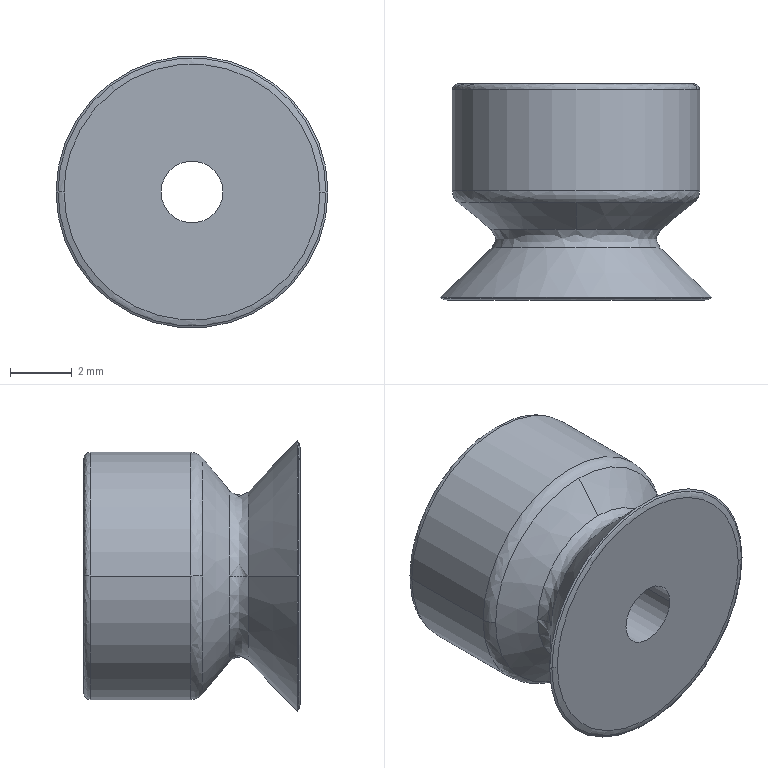Part | STEP file | 11-_ZP2-B08MUN_PADC11 | 1 solid | 20 faces | box 8.8 x 7 x 8.8 mm | volume 283.623 mm3 | spline 8 | cone 6 | cylinder 4 | plane 2 | commonest cylinder face diameters 2 x2 8 x2
STEP:
#1=CARTESIAN_POINT('',(0.,3.15,-3.815));
#2=VERTEX_POINT('',#1);
#3=CARTESIAN_POINT('',(-3.815,3.15,0.));
#4=VERTEX_POINT('',#3);
#5=CARTESIAN_POINT('',(0.,3.15,0.));
#6=DIRECTION('',(0.,1.,0.));
#7=DIRECTION('',(1.,0.,0.));
#8=AXIS2_PLACEMENT_3D('',#5,#6,#7);
#9=CIRCLE('',#8,3.815);
#10=EDGE_CURVE('',#2,#4,#9,.T.);
#11=ORIENTED_EDGE('',*,*,#10,.T.);
#12=CARTESIAN_POINT('',(-4.,3.538,0.));
#13=VERTEX_POINT('',#12);
#14=CARTESIAN_POINT('',(-3.5,3.538,0.));
#15=DIRECTION('',(0.,0.,-1.));
#16=DIRECTION('',(-1.,0.,0.));
#17=AXIS2_PLACEMENT_3D('',#14,#15,#16);
#18=CIRCLE('',#17,0.5);
#19=EDGE_CURVE('',#4,#13,#18,.T.);
#20=ORIENTED_EDGE('',*,*,#19,.T.);
#21=CARTESIAN_POINT('',(4.,3.538,0.));
#22=VERTEX_POINT('',#21);
#23=CARTESIAN_POINT('',(0.,3.538,0.));
#24=DIRECTION('',(0.,1.,0.));
#25=DIRECTION('',(-1.,0.,0.));
#26=AXIS2_PLACEMENT_3D('',#23,#24,#25);
#27=CIRCLE('',#26,4.);
#28=EDGE_CURVE('',#22,#13,#27,.T.);
#29=ORIENTED_EDGE('',*,*,#28,.F.);
#30=CARTESIAN_POINT('',(3.815,3.15,0.));
#31=VERTEX_POINT('',#30);
#32=CARTESIAN_POINT('',(3.5,3.538,0.));
#33=DIRECTION('',(0.,0.,1.));
#34=DIRECTION('',(1.,0.,0.));
#35=AXIS2_PLACEMENT_3D('',#32,#33,#34);
#36=CIRCLE('',#35,0.5);
#37=EDGE_CURVE('',#31,#22,#36,.T.);
#38=ORIENTED_EDGE('',*,*,#37,.F.);
#39=CARTESIAN_POINT('',(0.,3.15,0.));
#40=DIRECTION('',(0.,1.,0.));
#41=DIRECTION('',(1.,0.,0.));
#42=AXIS2_PLACEMENT_3D('',#39,#40,#41);
#43=CIRCLE('',#42,3.815);
#44=EDGE_CURVE('',#31,#2,#43,.T.);
#45=ORIENTED_EDGE('',*,*,#44,.T.);
#46=EDGE_LOOP('',(#11,#20,#29,#38,#45));
#47=FACE_OUTER_BOUND('',#46,.T.);
#48=CARTESIAN_POINT('',(-3.815,3.15,0.));
#49=CARTESIAN_POINT('',(-3.815,3.15,-7.631));
#50=CARTESIAN_POINT('',(3.815,3.15,-7.631));
#51=CARTESIAN_POINT('',(3.815,3.15,0.));
#52=CARTESIAN_POINT('',(-3.934,3.247,0.));
#53=CARTESIAN_POINT('',(-3.934,3.247,-7.868));
#54=CARTESIAN_POINT('',(3.934,3.247,-7.868));
#55=CARTESIAN_POINT('',(3.934,3.247,0.));
#56=CARTESIAN_POINT('',(-4.,3.385,0.));
#57=CARTESIAN_POINT('',(-4.,3.385,-8.));
#58=CARTESIAN_POINT('',(4.,3.385,-8.));
#59=CARTESIAN_POINT('',(4.,3.385,0.));
#60=CARTESIAN_POINT('',(-4.,3.538,0.));
#61=CARTESIAN_POINT('',(-4.,3.538,-8.));
#62=CARTESIAN_POINT('',(4.,3.538,-8.));
#63=CARTESIAN_POINT('',(4.,3.538,0.));
#64=(BOUNDED_SURFACE()B_SPLINE_SURFACE(3,3,((#48,#49,#50,#51),(#52,#53,#54,#55),(#56,#57,#58,#59),(#60,#61,#62,#63)),.UNSPECIFIED.,.F.,.F.,.F.)B_SPLINE_SURFACE_WITH_KNOTS((4,4),(4,4),(0.,1.),(0.,1.),.UNSPECIFIED.)GEOMETRIC_REPRESENTATION_ITEM()RATIONAL_B_SPLINE_SURFACE(((1.,0.3333,0.3333,1.),(0.9353,0.3118,0.3118,0.9353),(0.9353,0.3118,0.3118,0.9353),(1.,0.3333,0.3333,1.)))REPRESENTATION_ITEM('')SURFACE());
#65=ADVANCED_FACE('',(#47),#64,.T.);
#66=CARTESIAN_POINT('',(-4.,6.8,0.));
#67=VERTEX_POINT('',#66);
#68=CARTESIAN_POINT('',(4.,6.8,0.));
#69=VERTEX_POINT('',#68);
#70=CARTESIAN_POINT('',(0.,6.8,0.));
#71=DIRECTION('',(0.,-1.,0.));
#72=DIRECTION('',(-1.,0.,0.));
#73=AXIS2_PLACEMENT_3D('',#70,#71,#72);
#74=CIRCLE('',#73,4.);
#75=EDGE_CURVE('',#67,#69,#74,.T.);
#76=ORIENTED_EDGE('',*,*,#75,.F.);
#77=CARTESIAN_POINT('',(-3.8,7.,0.));
#78=VERTEX_POINT('',#77);
#79=CARTESIAN_POINT('',(-3.8,6.8,0.));
#80=DIRECTION('',(0.,0.,-1.));
#81=DIRECTION('',(-1.,0.,0.));
#82=AXIS2_PLACEMENT_3D('',#79,#80,#81);
#83=CIRCLE('',#82,0.2);
#84=EDGE_CURVE('',#67,#78,#83,.T.);
#85=ORIENTED_EDGE('',*,*,#84,.T.);
#86=CARTESIAN_POINT('',(3.8,7.,0.));
#87=VERTEX_POINT('',#86);
#88=CARTESIAN_POINT('',(-3.8,7.,0.));
#89=CARTESIAN_POINT('',(-3.8,7.,-7.6));
#90=CARTESIAN_POINT('',(3.8,7.,-7.6));
#91=CARTESIAN_POINT('',(3.8,7.,0.));
#92=(BOUNDED_CURVE()B_SPLINE_CURVE(3,(#88,#89,#90,#91),.UNSPECIFIED.,.F.,.F.)B_SPLINE_CURVE_WITH_KNOTS((4,4),(0.5,1.),.UNSPECIFIED.)CURVE()GEOMETRIC_REPRESENTATION_ITEM()RATIONAL_B_SPLINE_CURVE((1.,0.3333,0.3333,1.))REPRESENTATION_ITEM(''));
#93=EDGE_CURVE('',#78,#87,#92,.T.);
#94=ORIENTED_EDGE('',*,*,#93,.T.);
#95=CARTESIAN_POINT('',(3.8,6.8,0.));
#96=DIRECTION('',(0.,0.,1.));
#97=DIRECTION('',(1.,0.,0.));
#98=AXIS2_PLACEMENT_3D('',#95,#96,#97);
#99=CIRCLE('',#98,0.2);
#100=EDGE_CURVE('',#69,#87,#99,.T.);
#101=ORIENTED_EDGE('',*,*,#100,.F.);
#102=EDGE_LOOP('',(#76,#85,#94,#101));
#103=FACE_OUTER_BOUND('',#102,.T.);
#104=CARTESIAN_POINT('',(-4.,6.8,0.));
#105=CARTESIAN_POINT('',(-4.,6.8,-8.));
#106=CARTESIAN_POINT('',(4.,6.8,-8.));
#107=CARTESIAN_POINT('',(4.,6.8,0.));
#108=CARTESIAN_POINT('',(-4.,6.917,0.));
#109=CARTESIAN_POINT('',(-4.,6.917,-8.));
#110=CARTESIAN_POINT('',(4.,6.917,-8.));
#111=CARTESIAN_POINT('',(4.,6.917,0.));
#112=CARTESIAN_POINT('',(-3.917,7.,0.));
#113=CARTESIAN_POINT('',(-3.917,7.,-7.834));
#114=CARTESIAN_POINT('',(3.917,7.,-7.834));
#115=CARTESIAN_POINT('',(3.917,7.,0.));
#116=CARTESIAN_POINT('',(-3.8,7.,0.));
#117=CARTESIAN_POINT('',(-3.8,7.,-7.6));
#118=CARTESIAN_POINT('',(3.8,7.,-7.6));
#119=CARTESIAN_POINT('',(3.8,7.,0.));
#120=(BOUNDED_SURFACE()B_SPLINE_SURFACE(3,3,((#104,#105,#106,#107),(#108,#109,#110,#111),(#112,#113,#114,#115),(#116,#117,#118,#119)),.UNSPECIFIED.,.F.,.F.,.F.)B_SPLINE_SURFACE_WITH_KNOTS((4,4),(4,4),(0.,1.),(0.,1.),.UNSPECIFIED.)GEOMETRIC_REPRESENTATION_ITEM()RATIONAL_B_SPLINE_SURFACE(((1.,0.3333,0.3333,1.),(0.8047,0.2682,0.2682,0.8047),(0.8047,0.2682,0.2682,0.8047),(1.,0.3333,0.3333,1.)))REPRESENTATION_ITEM('')SURFACE());
#121=ADVANCED_FACE('',(#103),#120,.T.);
#122=CARTESIAN_POINT('',(-2.752,2.286,0.));
#123=VERTEX_POINT('',#122);
#124=CARTESIAN_POINT('',(0.,2.286,2.752));
#125=VERTEX_POINT('',#124);
#126=CARTESIAN_POINT('',(0.,2.286,0.));
#127=DIRECTION('',(0.,1.,0.));
#128=DIRECTION('',(-1.,0.,0.));
#129=AXIS2_PLACEMENT_3D('',#126,#127,#128);
#130=CIRCLE('',#129,2.752);
#131=EDGE_CURVE('',#123,#125,#130,.T.);
#132=ORIENTED_EDGE('',*,*,#131,.F.);
#133=CARTESIAN_POINT('',(-2.728,1.687,0.));
#134=VERTEX_POINT('',#133);
#135=CARTESIAN_POINT('',(-3.005,1.976,0.));
#136=DIRECTION('',(0.,0.,-1.));
#137=DIRECTION('',(-1.,0.,0.));
#138=AXIS2_PLACEMENT_3D('',#135,#136,#137);
#139=CIRCLE('',#138,0.4);
#140=EDGE_CURVE('',#123,#134,#139,.T.);
#141=ORIENTED_EDGE('',*,*,#140,.T.);
#142=CARTESIAN_POINT('',(2.728,1.687,0.));
#143=VERTEX_POINT('',#142);
#144=CARTESIAN_POINT('',(0.,1.687,0.));
#145=DIRECTION('',(0.,-1.,0.));
#146=DIRECTION('',(1.,0.,0.));
#147=AXIS2_PLACEMENT_3D('',#144,#145,#146);
#148=CIRCLE('',#147,2.728);
#149=EDGE_CURVE('',#143,#134,#148,.T.);
#150=ORIENTED_EDGE('',*,*,#149,.F.);
#151=CARTESIAN_POINT('',(2.752,2.286,0.));
#152=VERTEX_POINT('',#151);
#153=CARTESIAN_POINT('',(3.005,1.976,0.));
#154=DIRECTION('',(0.,0.,1.));
#155=DIRECTION('',(1.,0.,0.));
#156=AXIS2_PLACEMENT_3D('',#153,#154,#155);
#157=CIRCLE('',#156,0.4);
#158=EDGE_CURVE('',#152,#143,#157,.T.);
#159=ORIENTED_EDGE('',*,*,#158,.F.);
#160=CARTESIAN_POINT('',(0.,2.286,0.));
#161=DIRECTION('',(0.,1.,0.));
#162=DIRECTION('',(-1.,0.,0.));
#163=AXIS2_PLACEMENT_3D('',#160,#161,#162);
#164=CIRCLE('',#163,2.752);
#165=EDGE_CURVE('',#125,#152,#164,.T.);
#166=ORIENTED_EDGE('',*,*,#165,.F.);
#167=EDGE_LOOP('',(#132,#141,#150,#159,#166));
#168=FACE_OUTER_BOUND('',#167,.T.);
#169=CARTESIAN_POINT('',(2.752,2.286,0.));
#170=CARTESIAN_POINT('',(2.752,2.286,5.505));
#171=CARTESIAN_POINT('',(-2.752,2.286,5.505));
#172=CARTESIAN_POINT('',(-2.752,2.286,0.));
#173=CARTESIAN_POINT('',(2.552,2.123,0.));
#174=CARTESIAN_POINT('',(2.552,2.123,5.103));
#175=CARTESIAN_POINT('',(-2.552,2.123,5.103));
#176=CARTESIAN_POINT('',(-2.552,2.123,0.));
#177=CARTESIAN_POINT('',(2.541,1.865,0.));
#178=CARTESIAN_POINT('',(2.541,1.865,5.083));
#179=CARTESIAN_POINT('',(-2.541,1.865,5.083));
#180=CARTESIAN_POINT('',(-2.541,1.865,0.));
#181=CARTESIAN_POINT('',(2.728,1.687,0.));
#182=CARTESIAN_POINT('',(2.728,1.687,5.457));
#183=CARTESIAN_POINT('',(-2.728,1.687,5.457));
#184=CARTESIAN_POINT('',(-2.728,1.687,0.));
#185=(BOUNDED_SURFACE()B_SPLINE_SURFACE(3,3,((#169,#170,#171,#172),(#173,#174,#175,#176),(#177,#178,#179,#180),(#181,#182,#183,#184)),.UNSPECIFIED.,.F.,.F.,.F.)B_SPLINE_SURFACE_WITH_KNOTS((4,4),(4,4),(0.,1.),(0.,1.),.UNSPECIFIED.)GEOMETRIC_REPRESENTATION_ITEM()RATIONAL_B_SPLINE_SURFACE(((1.,0.3333,0.3333,1.),(0.7741,0.258,0.258,0.7741),(0.7741,0.258,0.258,0.7741),(1.,0.3333,0.3333,1.)))REPRESENTATION_ITEM('')SURFACE());
#186=ADVANCED_FACE('',(#168),#185,.F.);
#187=CARTESIAN_POINT('',(-4.137,0.,0.));
#188=VERTEX_POINT('',#187);
#189=CARTESIAN_POINT('',(4.137,0.,0.));
#190=VERTEX_POINT('',#189);
#191=CARTESIAN_POINT('',(-4.137,0.,0.));
#192=CARTESIAN_POINT('',(-4.137,0.,-0.2629));
#193=CARTESIAN_POINT('',(-4.101,0.,-0.6503));
#194=CARTESIAN_POINT('',(-3.995,0.,-1.091));
#195=CARTESIAN_POINT('',(-3.926,0.,-1.308));
#196=CARTESIAN_POINT('',(-3.893,0.,-1.4));
#197=CARTESIAN_POINT('',(-3.87,0.,-1.462));
#198=CARTESIAN_POINT('',(-3.859,0.,-1.49));
#199=CARTESIAN_POINT('',(-3.795,0.,-1.653));
#200=CARTESIAN_POINT('',(-3.709,0.,-1.843));
#201=CARTESIAN_POINT('',(-3.608,0.,-2.025));
#202=CARTESIAN_POINT('',(-3.538,0.,-2.146));
#203=CARTESIAN_POINT('',(-3.502,0.,-2.204));
#204=CARTESIAN_POINT('',(-3.307,0.,-2.503));
#205=CARTESIAN_POINT('',(-3.127,0.,-2.724));
#206=CARTESIAN_POINT('',(-2.824,0.,-3.026));
#207=CARTESIAN_POINT('',(-2.666,0.,-3.169));
#208=CARTESIAN_POINT('',(-2.497,0.,-3.299));
#209=CARTESIAN_POINT('',(-2.382,0.,-3.383));
#210=CARTESIAN_POINT('',(-2.322,0.,-3.424));
#211=CARTESIAN_POINT('',(-2.147,0.,-3.539));
#212=CARTESIAN_POINT('',(-1.967,0.,-3.644));
#213=CARTESIAN_POINT('',(-1.748,0.,-3.751));
#214=CARTESIAN_POINT('',(-1.652,0.,-3.793));
#215=CARTESIAN_POINT('',(-1.588,0.,-3.82));
#216=CARTESIAN_POINT('',(-1.553,0.,-3.834));
#217=CARTESIAN_POINT('',(-1.034,0.,-4.04));
#218=CARTESIAN_POINT('',(-0.5257,0.,-4.137));
#219=CARTESIAN_POINT('',(0.2629,0.,-4.137));
#220=CARTESIAN_POINT('',(0.6503,0.,-4.101));
#221=CARTESIAN_POINT('',(1.091,0.,-3.995));
#222=CARTESIAN_POINT('',(1.308,0.,-3.926));
#223=CARTESIAN_POINT('',(1.4,0.,-3.893));
#224=CARTESIAN_POINT('',(1.462,0.,-3.87));
#225=CARTESIAN_POINT('',(1.49,0.,-3.859));
#226=CARTESIAN_POINT('',(1.653,0.,-3.795));
#227=CARTESIAN_POINT('',(1.843,0.,-3.709));
#228=CARTESIAN_POINT('',(2.025,0.,-3.608));
#229=CARTESIAN_POINT('',(2.146,0.,-3.538));
#230=CARTESIAN_POINT('',(2.204,0.,-3.502));
#231=CARTESIAN_POINT('',(2.503,0.,-3.307));
#232=CARTESIAN_POINT('',(2.724,0.,-3.127));
#233=CARTESIAN_POINT('',(3.026,0.,-2.824));
#234=CARTESIAN_POINT('',(3.169,0.,-2.666));
#235=CARTESIAN_POINT('',(3.299,0.,-2.497));
#236=CARTESIAN_POINT('',(3.383,0.,-2.382));
#237=CARTESIAN_POINT('',(3.424,0.,-2.322));
#238=CARTESIAN_POINT('',(3.539,0.,-2.147));
#239=CARTESIAN_POINT('',(3.644,0.,-1.967));
#240=CARTESIAN_POINT('',(3.751,0.,-1.748));
#241=CARTESIAN_POINT('',(3.793,0.,-1.652));
#242=CARTESIAN_POINT('',(3.82,0.,-1.588));
#243=CARTESIAN_POINT('',(3.834,0.,-1.553));
#244=CARTESIAN_POINT('',(4.04,0.,-1.034));
#245=CARTESIAN_POINT('',(4.137,0.,-0.5262));
#246=CARTESIAN_POINT('',(4.137,0.,0.));
#247=B_SPLINE_CURVE_WITH_KNOTS('',3,(#191,#192,#193,#194,#195,#196,#197,#198,#199,#200,#201,#202,#203,#204,#205,#206,#207,#208,#209,#210,#211,#212,#213,#214,#215,#216,#217,#218,#219,#220,#221,#222,#223,#224,#225,#226,#227,#228,#229,#230,#231,#232,#233,#234,#235,#236,#237,#238,#239,#240,#241,#242,#243,#244,#245,#246),.UNSPECIFIED.,.F.,.F.,(4,1,1,1,2,2,1,2,2,2,1,2,2,1,1,2,2,2,1,1,1,2,2,1,2,2,2,1,2,2,1,1,2,2,4),(0.5,0.5313,0.5469,0.5547,0.5586,0.5625,0.5781,0.5859,0.5938,0.625,0.6406,0.6484,0.6562,0.6719,0.6797,0.6836,0.6875,0.75,0.7813,0.7969,0.8047,0.8086,0.8125,0.8281,0.8359,0.8438,0.875,0.8906,0.8984,0.9063,0.9219,0.9297,0.9336,0.9375,1.),.UNSPECIFIED.);
#248=EDGE_CURVE('',#188,#190,#247,.T.);
#249=ORIENTED_EDGE('',*,*,#248,.F.);
#250=CARTESIAN_POINT('',(-4.337,0.05359,0.));
#251=VERTEX_POINT('',#250);
#252=CARTESIAN_POINT('',(-4.137,0.4,0.));
#253=DIRECTION('',(0.,0.,-1.));
#254=DIRECTION('',(-1.,0.,0.));
#255=AXIS2_PLACEMENT_3D('',#252,#253,#254);
#256=CIRCLE('',#255,0.4);
#257=EDGE_CURVE('',#188,#251,#256,.T.);
#258=ORIENTED_EDGE('',*,*,#257,.T.);
#259=CARTESIAN_POINT('',(4.337,0.05359,0.));
#260=VERTEX_POINT('',#259);
#261=CARTESIAN_POINT('',(0.,0.05359,0.));
#262=DIRECTION('',(0.,1.,0.));
#263=DIRECTION('',(-1.,0.,0.));
#264=AXIS2_PLACEMENT_3D('',#261,#262,#263);
#265=CIRCLE('',#264,4.337);
#266=EDGE_CURVE('',#260,#251,#265,.T.);
#267=ORIENTED_EDGE('',*,*,#266,.F.);
#268=CARTESIAN_POINT('',(4.137,0.4,0.));
#269=DIRECTION('',(0.,0.,1.));
#270=DIRECTION('',(1.,0.,0.));
#271=AXIS2_PLACEMENT_3D('',#268,#269,#270);
#272=CIRCLE('',#271,0.4);
#273=EDGE_CURVE('',#190,#260,#272,.T.);
#274=ORIENTED_EDGE('',*,*,#273,.F.);
#275=EDGE_LOOP('',(#249,#258,#267,#274));
#276=FACE_OUTER_BOUND('',#275,.T.);
#277=CARTESIAN_POINT('',(-4.137,0.,0.));
#278=CARTESIAN_POINT('',(-4.137,0.,-8.274));
#279=CARTESIAN_POINT('',(4.137,0.,-8.274));
#280=CARTESIAN_POINT('',(4.137,0.,0.));
#281=CARTESIAN_POINT('',(-4.208,0.,0.));
#282=CARTESIAN_POINT('',(-4.208,0.,-8.415));
#283=CARTESIAN_POINT('',(4.208,0.,-8.415));
#284=CARTESIAN_POINT('',(4.208,0.,0.));
#285=CARTESIAN_POINT('',(-4.276,0.01828,0.));
#286=CARTESIAN_POINT('',(-4.276,0.01828,-8.552));
#287=CARTESIAN_POINT('',(4.276,0.01828,-8.552));
#288=CARTESIAN_POINT('',(4.276,0.01828,0.));
#289=CARTESIAN_POINT('',(-4.337,0.05359,0.));
#290=CARTESIAN_POINT('',(-4.337,0.05359,-8.674));
#291=CARTESIAN_POINT('',(4.337,0.05359,-8.674));
#292=CARTESIAN_POINT('',(4.337,0.05359,0.));
#293=(BOUNDED_SURFACE()B_SPLINE_SURFACE(3,3,((#277,#278,#279,#280),(#281,#282,#283,#284),(#285,#286,#287,#288),(#289,#290,#291,#292)),.UNSPECIFIED.,.F.,.F.,.F.)B_SPLINE_SURFACE_WITH_KNOTS((4,4),(4,4),(0.,1.),(0.,1.),.UNSPECIFIED.)GEOMETRIC_REPRESENTATION_ITEM()RATIONAL_B_SPLINE_SURFACE(((1.,0.3333,0.3333,1.),(0.9773,0.3258,0.3258,0.9773),(0.9773,0.3258,0.3258,0.9773),(1.,0.3333,0.3333,1.)))REPRESENTATION_ITEM('')SURFACE());
#294=ADVANCED_FACE('',(#276),#293,.T.);
#295=CARTESIAN_POINT('',(0.,3.538,0.));
#296=DIRECTION('',(0.,1.,0.));
#297=DIRECTION('',(-1.,0.,0.));
#298=AXIS2_PLACEMENT_3D('',#295,#296,#297);
#299=CIRCLE('',#298,4.);
#300=EDGE_CURVE('',#13,#22,#299,.T.);
#301=ORIENTED_EDGE('',*,*,#300,.T.);
#302=CARTESIAN_POINT('',(4.,0.,0.));
#303=DIRECTION('',(0.,1.,0.));
#304=VECTOR('',#303,1000.);
#305=LINE('',#302,#304);
#306=EDGE_CURVE('',#22,#69,#305,.T.);
#307=ORIENTED_EDGE('',*,*,#306,.T.);
#308=CARTESIAN_POINT('',(0.,6.8,0.));
#309=DIRECTION('',(0.,-1.,0.));
#310=DIRECTION('',(-1.,0.,0.));
#311=AXIS2_PLACEMENT_3D('',#308,#309,#310);
#312=CIRCLE('',#311,4.);
#313=EDGE_CURVE('',#69,#67,#312,.T.);
#314=ORIENTED_EDGE('',*,*,#313,.T.);
#315=CARTESIAN_POINT('',(-4.,0.,0.));
#316=DIRECTION('',(0.,1.,0.));
#317=VECTOR('',#316,1000.);
#318=LINE('',#315,#317);
#319=EDGE_CURVE('',#13,#67,#318,.T.);
#320=ORIENTED_EDGE('',*,*,#319,.F.);
#321=EDGE_LOOP('',(#301,#307,#314,#320));
#322=FACE_OUTER_BOUND('',#321,.T.);
#323=CARTESIAN_POINT('',(0.,0.,0.));
#324=DIRECTION('',(0.,1.,0.));
#325=DIRECTION('',(-1.,0.,0.));
#326=AXIS2_PLACEMENT_3D('',#323,#324,#325);
#327=CYLINDRICAL_SURFACE('',#326,4.);
#328=ADVANCED_FACE('',(#322),#327,.T.);
#329=ORIENTED_EDGE('',*,*,#165,.T.);
#330=CARTESIAN_POINT('',(0.,2.286,-2.752));
#331=VERTEX_POINT('',#330);
#332=CARTESIAN_POINT('',(0.,2.286,0.));
#333=DIRECTION('',(0.,1.,0.));
#334=DIRECTION('',(-1.,0.,0.));
#335=AXIS2_PLACEMENT_3D('',#332,#333,#334);
#336=CIRCLE('',#335,2.752);
#337=EDGE_CURVE('',#152,#331,#336,.T.);
#338=ORIENTED_EDGE('',*,*,#337,.T.);
#339=CARTESIAN_POINT('',(0.,3.15,-3.815));
#340=DIRECTION('',(0.,0.6306,-0.7761));
#341=VECTOR('',#340,1000.);
#342=LINE('',#339,#341);
#343=EDGE_CURVE('',#331,#2,#342,.T.);
#344=ORIENTED_EDGE('',*,*,#343,.T.);
#345=ORIENTED_EDGE('',*,*,#44,.F.);
#346=CARTESIAN_POINT('',(0.,3.15,3.815));
#347=VERTEX_POINT('',#346);
#348=CARTESIAN_POINT('',(0.,3.15,0.));
#349=DIRECTION('',(0.,1.,0.));
#350=DIRECTION('',(1.,0.,0.));
#351=AXIS2_PLACEMENT_3D('',#348,#349,#350);
#352=CIRCLE('',#351,3.815);
#353=EDGE_CURVE('',#347,#31,#352,.T.);
#354=ORIENTED_EDGE('',*,*,#353,.F.);
#355=CARTESIAN_POINT('',(0.,3.15,3.815));
#356=DIRECTION('',(0.,0.6306,0.7761));
#357=VECTOR('',#356,1000.);
#358=LINE('',#355,#357);
#359=EDGE_CURVE('',#125,#347,#358,.T.);
#360=ORIENTED_EDGE('',*,*,#359,.F.);
#361=EDGE_LOOP('',(#329,#338,#344,#345,#354,#360));
#362=FACE_OUTER_BOUND('',#361,.T.);
#363=CARTESIAN_POINT('',(0.,3.15,0.));
#364=DIRECTION('',(0.,1.,0.));
#365=DIRECTION('',(0.,0.,1.));
#366=AXIS2_PLACEMENT_3D('',#363,#364,#365);
#367=CONICAL_SURFACE('',#366,3.815,0.8885);
#368=ADVANCED_FACE('',(#362),#367,.T.);
#369=CARTESIAN_POINT('',(1.,0.,0.));
#370=VERTEX_POINT('',#369);
#371=CARTESIAN_POINT('',(-1.,0.,0.));
#372=VERTEX_POINT('',#371);
#373=CARTESIAN_POINT('',(0.,0.,0.));
#374=DIRECTION('',(0.,1.,0.));
#375=DIRECTION('',(-1.,0.,0.));
#376=AXIS2_PLACEMENT_3D('',#373,#374,#375);
#377=CIRCLE('',#376,1.);
#378=EDGE_CURVE('',#370,#372,#377,.T.);
#379=ORIENTED_EDGE('',*,*,#378,.F.);
#380=CARTESIAN_POINT('',(1.,7.,0.));
#381=VERTEX_POINT('',#380);
#382=CARTESIAN_POINT('',(1.,0.,0.));
#383=DIRECTION('',(0.,1.,0.));
#384=VECTOR('',#383,1000.);
#385=LINE('',#382,#384);
#386=EDGE_CURVE('',#370,#381,#385,.T.);
#387=ORIENTED_EDGE('',*,*,#386,.T.);
#388=CARTESIAN_POINT('',(-1.,7.,0.));
#389=VERTEX_POINT('',#388);
#390=CARTESIAN_POINT('',(0.,7.,0.));
#391=DIRECTION('',(0.,-1.,0.));
#392=DIRECTION('',(-1.,0.,0.));
#393=AXIS2_PLACEMENT_3D('',#390,#391,#392);
#394=CIRCLE('',#393,1.);
#395=EDGE_CURVE('',#389,#381,#394,.T.);
#396=ORIENTED_EDGE('',*,*,#395,.F.);
#397=CARTESIAN_POINT('',(-1.,0.,0.));
#398=DIRECTION('',(0.,1.,0.));
#399=VECTOR('',#398,1000.);
#400=LINE('',#397,#399);
#401=EDGE_CURVE('',#372,#389,#400,.T.);
#402=ORIENTED_EDGE('',*,*,#401,.F.);
#403=EDGE_LOOP('',(#379,#387,#396,#402));
#404=FACE_OUTER_BOUND('',#403,.T.);
#405=CARTESIAN_POINT('',(0.,0.,0.));
#406=DIRECTION('',(0.,1.,0.));
#407=DIRECTION('',(-1.,0.,0.));
#408=AXIS2_PLACEMENT_3D('',#405,#406,#407);
#409=CYLINDRICAL_SURFACE('',#408,1.);
#410=ADVANCED_FACE('',(#404),#409,.F.);
#411=ORIENTED_EDGE('',*,*,#149,.T.);
#412=CARTESIAN_POINT('',(-4.4,0.09,0.));
#413=VERTEX_POINT('',#412);
#414=CARTESIAN_POINT('',(-4.4,0.09,0.));
#415=DIRECTION('',(-0.7232,-0.6906,0.));
#416=VECTOR('',#415,1000.);
#417=LINE('',#414,#416);
#418=EDGE_CURVE('',#134,#413,#417,.T.);
#419=ORIENTED_EDGE('',*,*,#418,.T.);
#420=CARTESIAN_POINT('',(4.4,0.09,0.));
#421=VERTEX_POINT('',#420);
#422=CARTESIAN_POINT('',(0.,0.09,0.));
#423=DIRECTION('',(0.,1.,0.));
#424=DIRECTION('',(1.,0.,0.));
#425=AXIS2_PLACEMENT_3D('',#422,#423,#424);
#426=CIRCLE('',#425,4.4);
#427=EDGE_CURVE('',#413,#421,#426,.T.);
#428=ORIENTED_EDGE('',*,*,#427,.T.);
#429=CARTESIAN_POINT('',(4.4,0.09,0.));
#430=DIRECTION('',(0.7232,-0.6906,0.));
#431=VECTOR('',#430,1000.);
#432=LINE('',#429,#431);
#433=EDGE_CURVE('',#143,#421,#432,.T.);
#434=ORIENTED_EDGE('',*,*,#433,.F.);
#435=EDGE_LOOP('',(#411,#419,#428,#434));
#436=FACE_OUTER_BOUND('',#435,.T.);
#437=CARTESIAN_POINT('',(0.,0.09,0.));
#438=DIRECTION('',(0.,-1.,0.));
#439=DIRECTION('',(1.,0.,0.));
#440=AXIS2_PLACEMENT_3D('',#437,#438,#439);
#441=CONICAL_SURFACE('',#440,4.4,0.8084);
#442=ADVANCED_FACE('',(#436),#441,.T.);
#443=CARTESIAN_POINT('',(0.,0.05359,0.));
#444=DIRECTION('',(0.,1.,0.));
#445=DIRECTION('',(-1.,0.,0.));
#446=AXIS2_PLACEMENT_3D('',#443,#444,#445);
#447=CIRCLE('',#446,4.337);
#448=EDGE_CURVE('',#251,#260,#447,.T.);
#449=ORIENTED_EDGE('',*,*,#448,.T.);
#450=CARTESIAN_POINT('',(4.4,0.09,0.));
#451=DIRECTION('',(0.866,0.5,0.));
#452=VECTOR('',#451,1000.);
#453=LINE('',#450,#452);
#454=EDGE_CURVE('',#260,#421,#453,.T.);
#455=ORIENTED_EDGE('',*,*,#454,.T.);
#456=ORIENTED_EDGE('',*,*,#427,.F.);
#457=CARTESIAN_POINT('',(-4.4,0.09,0.));
#458=DIRECTION('',(-0.866,0.5,0.));
#459=VECTOR('',#458,1000.);
#460=LINE('',#457,#459);
#461=EDGE_CURVE('',#251,#413,#460,.T.);
#462=ORIENTED_EDGE('',*,*,#461,.F.);
#463=EDGE_LOOP('',(#449,#455,#456,#462));
#464=FACE_OUTER_BOUND('',#463,.T.);
#465=CARTESIAN_POINT('',(0.,0.09,0.));
#466=DIRECTION('',(0.,1.,0.));
#467=DIRECTION('',(-1.,0.,0.));
#468=AXIS2_PLACEMENT_3D('',#465,#466,#467);
#469=CONICAL_SURFACE('',#468,4.4,1.047);
#470=ADVANCED_FACE('',(#464),#469,.T.);
#471=ORIENTED_EDGE('',*,*,#306,.F.);
#472=ORIENTED_EDGE('',*,*,#28,.T.);
#473=ORIENTED_EDGE('',*,*,#319,.T.);
#474=ORIENTED_EDGE('',*,*,#75,.T.);
#475=EDGE_LOOP('',(#471,#472,#473,#474));
#476=FACE_OUTER_BOUND('',#475,.T.);
#477=CARTESIAN_POINT('',(0.,0.,0.));
#478=DIRECTION('',(0.,1.,0.));
#479=DIRECTION('',(-1.,0.,0.));
#480=AXIS2_PLACEMENT_3D('',#477,#478,#479);
#481=CYLINDRICAL_SURFACE('',#480,4.);
#482=ADVANCED_FACE('',(#476),#481,.T.);
#483=ORIENTED_EDGE('',*,*,#19,.F.);
#484=CARTESIAN_POINT('',(0.,3.15,0.));
#485=DIRECTION('',(0.,1.,0.));
#486=DIRECTION('',(1.,0.,0.));
#487=AXIS2_PLACEMENT_3D('',#484,#485,#486);
#488=CIRCLE('',#487,3.815);
#489=EDGE_CURVE('',#4,#347,#488,.T.);
#490=ORIENTED_EDGE('',*,*,#489,.T.);
#491=ORIENTED_EDGE('',*,*,#353,.T.);
#492=ORIENTED_EDGE('',*,*,#37,.T.);
#493=ORIENTED_EDGE('',*,*,#300,.F.);
#494=EDGE_LOOP('',(#483,#490,#491,#492,#493));
#495=FACE_OUTER_BOUND('',#494,.T.);
#496=CARTESIAN_POINT('',(3.815,3.15,0.));
#497=CARTESIAN_POINT('',(3.815,3.15,7.631));
#498=CARTESIAN_POINT('',(-3.815,3.15,7.631));
#499=CARTESIAN_POINT('',(-3.815,3.15,0.));
#500=CARTESIAN_POINT('',(3.934,3.247,0.));
#501=CARTESIAN_POINT('',(3.934,3.247,7.868));
#502=CARTESIAN_POINT('',(-3.934,3.247,7.868));
#503=CARTESIAN_POINT('',(-3.934,3.247,0.));
#504=CARTESIAN_POINT('',(4.,3.385,0.));
#505=CARTESIAN_POINT('',(4.,3.385,8.));
#506=CARTESIAN_POINT('',(-4.,3.385,8.));
#507=CARTESIAN_POINT('',(-4.,3.385,0.));
#508=CARTESIAN_POINT('',(4.,3.538,0.));
#509=CARTESIAN_POINT('',(4.,3.538,8.));
#510=CARTESIAN_POINT('',(-4.,3.538,8.));
#511=CARTESIAN_POINT('',(-4.,3.538,0.));
#512=(BOUNDED_SURFACE()B_SPLINE_SURFACE(3,3,((#496,#497,#498,#499),(#500,#501,#502,#503),(#504,#505,#506,#507),(#508,#509,#510,#511)),.UNSPECIFIED.,.F.,.F.,.F.)B_SPLINE_SURFACE_WITH_KNOTS((4,4),(4,4),(0.,1.),(0.,1.),.UNSPECIFIED.)GEOMETRIC_REPRESENTATION_ITEM()RATIONAL_B_SPLINE_SURFACE(((1.,0.3333,0.3333,1.),(0.9353,0.3118,0.3118,0.9353),(0.9353,0.3118,0.3118,0.9353),(1.,0.3333,0.3333,1.)))REPRESENTATION_ITEM('')SURFACE());
#513=ADVANCED_FACE('',(#495),#512,.T.);
#514=ORIENTED_EDGE('',*,*,#84,.F.);
#515=ORIENTED_EDGE('',*,*,#313,.F.);
#516=ORIENTED_EDGE('',*,*,#100,.T.);
#517=CARTESIAN_POINT('',(3.8,7.,0.));
#518=CARTESIAN_POINT('',(3.8,7.,7.6));
#519=CARTESIAN_POINT('',(-3.8,7.,7.6));
#520=CARTESIAN_POINT('',(-3.8,7.,0.));
#521=(BOUNDED_CURVE()B_SPLINE_CURVE(3,(#517,#518,#519,#520),.UNSPECIFIED.,.F.,.F.)B_SPLINE_CURVE_WITH_KNOTS((4,4),(0.,0.5),.UNSPECIFIED.)CURVE()GEOMETRIC_REPRESENTATION_ITEM()RATIONAL_B_SPLINE_CURVE((1.,0.3333,0.3333,1.))REPRESENTATION_ITEM(''));
#522=EDGE_CURVE('',#87,#78,#521,.T.);
#523=ORIENTED_EDGE('',*,*,#522,.T.);
#524=EDGE_LOOP('',(#514,#515,#516,#523));
#525=FACE_OUTER_BOUND('',#524,.T.);
#526=CARTESIAN_POINT('',(4.,6.8,0.));
#527=CARTESIAN_POINT('',(4.,6.8,8.));
#528=CARTESIAN_POINT('',(-4.,6.8,8.));
#529=CARTESIAN_POINT('',(-4.,6.8,0.));
#530=CARTESIAN_POINT('',(4.,6.917,0.));
#531=CARTESIAN_POINT('',(4.,6.917,8.));
#532=CARTESIAN_POINT('',(-4.,6.917,8.));
#533=CARTESIAN_POINT('',(-4.,6.917,0.));
#534=CARTESIAN_POINT('',(3.917,7.,0.));
#535=CARTESIAN_POINT('',(3.917,7.,7.834));
#536=CARTESIAN_POINT('',(-3.917,7.,7.834));
#537=CARTESIAN_POINT('',(-3.917,7.,0.));
#538=CARTESIAN_POINT('',(3.8,7.,0.));
#539=CARTESIAN_POINT('',(3.8,7.,7.6));
#540=CARTESIAN_POINT('',(-3.8,7.,7.6));
#541=CARTESIAN_POINT('',(-3.8,7.,0.));
#542=(BOUNDED_SURFACE()B_SPLINE_SURFACE(3,3,((#526,#527,#528,#529),(#530,#531,#532,#533),(#534,#535,#536,#537),(#538,#539,#540,#541)),.UNSPECIFIED.,.F.,.F.,.F.)B_SPLINE_SURFACE_WITH_KNOTS((4,4),(4,4),(0.,1.),(0.,1.),.UNSPECIFIED.)GEOMETRIC_REPRESENTATION_ITEM()RATIONAL_B_SPLINE_SURFACE(((1.,0.3333,0.3333,1.),(0.8047,0.2682,0.2682,0.8047),(0.8047,0.2682,0.2682,0.8047),(1.,0.3333,0.3333,1.)))REPRESENTATION_ITEM('')SURFACE());
#543=ADVANCED_FACE('',(#525),#542,.T.);
#544=ORIENTED_EDGE('',*,*,#343,.F.);
#545=CARTESIAN_POINT('',(0.,2.286,0.));
#546=DIRECTION('',(0.,1.,0.));
#547=DIRECTION('',(-1.,0.,0.));
#548=AXIS2_PLACEMENT_3D('',#545,#546,#547);
#549=CIRCLE('',#548,2.752);
#550=EDGE_CURVE('',#331,#123,#549,.T.);
#551=ORIENTED_EDGE('',*,*,#550,.T.);
#552=ORIENTED_EDGE('',*,*,#131,.T.);
#553=ORIENTED_EDGE('',*,*,#359,.T.);
#554=ORIENTED_EDGE('',*,*,#489,.F.);
#555=ORIENTED_EDGE('',*,*,#10,.F.);
#556=EDGE_LOOP('',(#544,#551,#552,#553,#554,#555));
#557=FACE_OUTER_BOUND('',#556,.T.);
#558=CARTESIAN_POINT('',(0.,3.15,0.));
#559=DIRECTION('',(0.,1.,0.));
#560=DIRECTION('',(0.,0.,1.));
#561=AXIS2_PLACEMENT_3D('',#558,#559,#560);
#562=CONICAL_SURFACE('',#561,3.815,0.8885);
#563=ADVANCED_FACE('',(#557),#562,.T.);
#564=ORIENTED_EDGE('',*,*,#522,.F.);
#565=ORIENTED_EDGE('',*,*,#93,.F.);
#566=EDGE_LOOP('',(#564,#565));
#567=FACE_OUTER_BOUND('',#566,.T.);
#568=ORIENTED_EDGE('',*,*,#395,.T.);
#569=CARTESIAN_POINT('',(0.,7.,0.));
#570=DIRECTION('',(0.,-1.,0.));
#571=DIRECTION('',(-1.,0.,0.));
#572=AXIS2_PLACEMENT_3D('',#569,#570,#571);
#573=CIRCLE('',#572,1.);
#574=EDGE_CURVE('',#381,#389,#573,.T.);
#575=ORIENTED_EDGE('',*,*,#574,.T.);
#576=EDGE_LOOP('',(#568,#575));
#577=FACE_BOUND('',#576,.T.);
#578=CARTESIAN_POINT('',(3.8,7.,0.));
#579=DIRECTION('',(0.,1.,0.));
#580=DIRECTION('',(-1.,0.,0.));
#581=AXIS2_PLACEMENT_3D('',#578,#579,#580);
#582=PLANE('',#581);
#583=ADVANCED_FACE('',(#567,#577),#582,.T.);
#584=ORIENTED_EDGE('',*,*,#140,.F.);
#585=ORIENTED_EDGE('',*,*,#550,.F.);
#586=ORIENTED_EDGE('',*,*,#337,.F.);
#587=ORIENTED_EDGE('',*,*,#158,.T.);
#588=CARTESIAN_POINT('',(0.,1.687,0.));
#589=DIRECTION('',(0.,-1.,0.));
#590=DIRECTION('',(1.,0.,0.));
#591=AXIS2_PLACEMENT_3D('',#588,#589,#590);
#592=CIRCLE('',#591,2.728);
#593=EDGE_CURVE('',#134,#143,#592,.T.);
#594=ORIENTED_EDGE('',*,*,#593,.F.);
#595=EDGE_LOOP('',(#584,#585,#586,#587,#594));
#596=FACE_OUTER_BOUND('',#595,.T.);
#597=CARTESIAN_POINT('',(-2.752,2.286,0.));
#598=CARTESIAN_POINT('',(-2.752,2.286,-5.505));
#599=CARTESIAN_POINT('',(2.752,2.286,-5.505));
#600=CARTESIAN_POINT('',(2.752,2.286,0.));
#601=CARTESIAN_POINT('',(-2.552,2.123,0.));
#602=CARTESIAN_POINT('',(-2.552,2.123,-5.103));
#603=CARTESIAN_POINT('',(2.552,2.123,-5.103));
#604=CARTESIAN_POINT('',(2.552,2.123,0.));
#605=CARTESIAN_POINT('',(-2.541,1.865,0.));
#606=CARTESIAN_POINT('',(-2.541,1.865,-5.083));
#607=CARTESIAN_POINT('',(2.541,1.865,-5.083));
#608=CARTESIAN_POINT('',(2.541,1.865,0.));
#609=CARTESIAN_POINT('',(-2.728,1.687,0.));
#610=CARTESIAN_POINT('',(-2.728,1.687,-5.457));
#611=CARTESIAN_POINT('',(2.728,1.687,-5.457));
#612=CARTESIAN_POINT('',(2.728,1.687,0.));
#613=(BOUNDED_SURFACE()B_SPLINE_SURFACE(3,3,((#597,#598,#599,#600),(#601,#602,#603,#604),(#605,#606,#607,#608),(#609,#610,#611,#612)),.UNSPECIFIED.,.F.,.F.,.F.)B_SPLINE_SURFACE_WITH_KNOTS((4,4),(4,4),(0.,1.),(0.,1.),.UNSPECIFIED.)GEOMETRIC_REPRESENTATION_ITEM()RATIONAL_B_SPLINE_SURFACE(((1.,0.3333,0.3333,1.),(0.7741,0.258,0.258,0.7741),(0.7741,0.258,0.258,0.7741),(1.,0.3333,0.3333,1.)))REPRESENTATION_ITEM('')SURFACE());
#614=ADVANCED_FACE('',(#596),#613,.F.);
#615=ORIENTED_EDGE('',*,*,#386,.F.);
#616=CARTESIAN_POINT('',(0.,0.,0.));
#617=DIRECTION('',(0.,1.,0.));
#618=DIRECTION('',(-1.,0.,0.));
#619=AXIS2_PLACEMENT_3D('',#616,#617,#618);
#620=CIRCLE('',#619,1.);
#621=EDGE_CURVE('',#372,#370,#620,.T.);
#622=ORIENTED_EDGE('',*,*,#621,.F.);
#623=ORIENTED_EDGE('',*,*,#401,.T.);
#624=ORIENTED_EDGE('',*,*,#574,.F.);
#625=EDGE_LOOP('',(#615,#622,#623,#624));
#626=FACE_OUTER_BOUND('',#625,.T.);
#627=CARTESIAN_POINT('',(0.,0.,0.));
#628=DIRECTION('',(0.,1.,0.));
#629=DIRECTION('',(-1.,0.,0.));
#630=AXIS2_PLACEMENT_3D('',#627,#628,#629);
#631=CYLINDRICAL_SURFACE('',#630,1.);
#632=ADVANCED_FACE('',(#626),#631,.F.);
#633=ORIENTED_EDGE('',*,*,#418,.F.);
#634=ORIENTED_EDGE('',*,*,#593,.T.);
#635=ORIENTED_EDGE('',*,*,#433,.T.);
#636=CARTESIAN_POINT('',(0.,0.09,0.));
#637=DIRECTION('',(0.,1.,0.));
#638=DIRECTION('',(1.,0.,0.));
#639=AXIS2_PLACEMENT_3D('',#636,#637,#638);
#640=CIRCLE('',#639,4.4);
#641=EDGE_CURVE('',#421,#413,#640,.T.);
#642=ORIENTED_EDGE('',*,*,#641,.T.);
#643=EDGE_LOOP('',(#633,#634,#635,#642));
#644=FACE_OUTER_BOUND('',#643,.T.);
#645=CARTESIAN_POINT('',(0.,0.09,0.));
#646=DIRECTION('',(0.,-1.,0.));
#647=DIRECTION('',(1.,0.,0.));
#648=AXIS2_PLACEMENT_3D('',#645,#646,#647);
#649=CONICAL_SURFACE('',#648,4.4,0.8084);
#650=ADVANCED_FACE('',(#644),#649,.T.);
#651=ORIENTED_EDGE('',*,*,#621,.T.);
#652=ORIENTED_EDGE('',*,*,#378,.T.);
#653=EDGE_LOOP('',(#651,#652));
#654=FACE_BOUND('',#653,.T.);
#655=CARTESIAN_POINT('',(4.137,0.,0.));
#656=CARTESIAN_POINT('',(4.137,0.,0.2629));
#657=CARTESIAN_POINT('',(4.101,0.,0.6505));
#658=CARTESIAN_POINT('',(3.995,0.,1.091));
#659=CARTESIAN_POINT('',(3.926,0.,1.308));
#660=CARTESIAN_POINT('',(3.893,0.,1.4));
#661=CARTESIAN_POINT('',(3.87,0.,1.462));
#662=CARTESIAN_POINT('',(3.859,0.,1.49));
#663=CARTESIAN_POINT('',(3.795,0.,1.653));
#664=CARTESIAN_POINT('',(3.709,0.,1.843));
#665=CARTESIAN_POINT('',(3.608,0.,2.025));
#666=CARTESIAN_POINT('',(3.538,0.,2.146));
#667=CARTESIAN_POINT('',(3.502,0.,2.204));
#668=CARTESIAN_POINT('',(3.307,0.,2.503));
#669=CARTESIAN_POINT('',(3.127,0.,2.724));
#670=CARTESIAN_POINT('',(2.824,0.,3.026));
#671=CARTESIAN_POINT('',(2.666,0.,3.169));
#672=CARTESIAN_POINT('',(2.497,0.,3.299));
#673=CARTESIAN_POINT('',(2.382,0.,3.383));
#674=CARTESIAN_POINT('',(2.322,0.,3.424));
#675=CARTESIAN_POINT('',(2.147,0.,3.539));
#676=CARTESIAN_POINT('',(1.967,0.,3.644));
#677=CARTESIAN_POINT('',(1.748,0.,3.751));
#678=CARTESIAN_POINT('',(1.652,0.,3.793));
#679=CARTESIAN_POINT('',(1.588,0.,3.82));
#680=CARTESIAN_POINT('',(1.553,0.,3.834));
#681=CARTESIAN_POINT('',(1.034,0.,4.04));
#682=CARTESIAN_POINT('',(0.5257,0.,4.137));
#683=CARTESIAN_POINT('',(-0.2629,0.,4.137));
#684=CARTESIAN_POINT('',(-0.6503,0.,4.101));
#685=CARTESIAN_POINT('',(-1.091,0.,3.995));
#686=CARTESIAN_POINT('',(-1.308,0.,3.926));
#687=CARTESIAN_POINT('',(-1.4,0.,3.893));
#688=CARTESIAN_POINT('',(-1.462,0.,3.87));
#689=CARTESIAN_POINT('',(-1.49,0.,3.859));
#690=CARTESIAN_POINT('',(-1.653,0.,3.795));
#691=CARTESIAN_POINT('',(-1.843,0.,3.709));
#692=CARTESIAN_POINT('',(-2.025,0.,3.608));
#693=CARTESIAN_POINT('',(-2.146,0.,3.538));
#694=CARTESIAN_POINT('',(-2.204,0.,3.502));
#695=CARTESIAN_POINT('',(-2.503,0.,3.307));
#696=CARTESIAN_POINT('',(-2.724,0.,3.127));
#697=CARTESIAN_POINT('',(-3.026,0.,2.824));
#698=CARTESIAN_POINT('',(-3.169,0.,2.666));
#699=CARTESIAN_POINT('',(-3.299,0.,2.497));
#700=CARTESIAN_POINT('',(-3.383,0.,2.382));
#701=CARTESIAN_POINT('',(-3.424,0.,2.322));
#702=CARTESIAN_POINT('',(-3.539,0.,2.147));
#703=CARTESIAN_POINT('',(-3.644,0.,1.967));
#704=CARTESIAN_POINT('',(-3.751,0.,1.748));
#705=CARTESIAN_POINT('',(-3.793,0.,1.652));
#706=CARTESIAN_POINT('',(-3.82,0.,1.588));
#707=CARTESIAN_POINT('',(-3.834,0.,1.553));
#708=CARTESIAN_POINT('',(-4.04,0.,1.034));
#709=CARTESIAN_POINT('',(-4.137,0.,0.5257));
#710=CARTESIAN_POINT('',(-4.137,0.,0.));
#711=B_SPLINE_CURVE_WITH_KNOTS('',3,(#655,#656,#657,#658,#659,#660,#661,#662,#663,#664,#665,#666,#667,#668,#669,#670,#671,#672,#673,#674,#675,#676,#677,#678,#679,#680,#681,#682,#683,#684,#685,#686,#687,#688,#689,#690,#691,#692,#693,#694,#695,#696,#697,#698,#699,#700,#701,#702,#703,#704,#705,#706,#707,#708,#709,#710),.UNSPECIFIED.,.F.,.F.,(4,1,1,1,2,2,1,2,2,2,1,2,2,1,1,2,2,2,1,1,1,2,2,1,2,2,2,1,2,2,1,1,2,2,4),(0.,0.03125,0.04688,0.05469,0.05859,0.0625,0.07813,0.08594,0.09375,0.125,0.1406,0.1484,0.1563,0.1719,0.1797,0.1836,0.1875,0.25,0.2813,0.2969,0.3047,0.3086,0.3125,0.3281,0.3359,0.3438,0.375,0.3906,0.3984,0.4063,0.4219,0.4297,0.4336,0.4375,0.5),.UNSPECIFIED.);
#712=EDGE_CURVE('',#190,#188,#711,.T.);
#713=ORIENTED_EDGE('',*,*,#712,.T.);
#714=ORIENTED_EDGE('',*,*,#248,.T.);
#715=EDGE_LOOP('',(#713,#714));
#716=FACE_OUTER_BOUND('',#715,.T.);
#717=CARTESIAN_POINT('',(1.,0.,0.));
#718=DIRECTION('',(0.,-1.,0.));
#719=DIRECTION('',(1.,0.,0.));
#720=AXIS2_PLACEMENT_3D('',#717,#718,#719);
#721=PLANE('',#720);
#722=ADVANCED_FACE('',(#654,#716),#721,.T.);
#723=ORIENTED_EDGE('',*,*,#454,.F.);
#724=ORIENTED_EDGE('',*,*,#266,.T.);
#725=ORIENTED_EDGE('',*,*,#461,.T.);
#726=ORIENTED_EDGE('',*,*,#641,.F.);
#727=EDGE_LOOP('',(#723,#724,#725,#726));
#728=FACE_OUTER_BOUND('',#727,.T.);
#729=CARTESIAN_POINT('',(0.,0.09,0.));
#730=DIRECTION('',(0.,1.,0.));
#731=DIRECTION('',(-1.,0.,0.));
#732=AXIS2_PLACEMENT_3D('',#729,#730,#731);
#733=CONICAL_SURFACE('',#732,4.4,1.047);
#734=ADVANCED_FACE('',(#728),#733,.T.);
#735=ORIENTED_EDGE('',*,*,#257,.F.);
#736=ORIENTED_EDGE('',*,*,#712,.F.);
#737=ORIENTED_EDGE('',*,*,#273,.T.);
#738=ORIENTED_EDGE('',*,*,#448,.F.);
#739=EDGE_LOOP('',(#735,#736,#737,#738));
#740=FACE_OUTER_BOUND('',#739,.T.);
#741=CARTESIAN_POINT('',(4.137,0.,0.));
#742=CARTESIAN_POINT('',(4.137,0.,8.274));
#743=CARTESIAN_POINT('',(-4.137,0.,8.274));
#744=CARTESIAN_POINT('',(-4.137,0.,0.));
#745=CARTESIAN_POINT('',(4.208,0.,0.));
#746=CARTESIAN_POINT('',(4.208,0.,8.415));
#747=CARTESIAN_POINT('',(-4.208,0.,8.415));
#748=CARTESIAN_POINT('',(-4.208,0.,0.));
#749=CARTESIAN_POINT('',(4.276,0.01828,0.));
#750=CARTESIAN_POINT('',(4.276,0.01828,8.552));
#751=CARTESIAN_POINT('',(-4.276,0.01828,8.552));
#752=CARTESIAN_POINT('',(-4.276,0.01828,0.));
#753=CARTESIAN_POINT('',(4.337,0.05359,0.));
#754=CARTESIAN_POINT('',(4.337,0.05359,8.674));
#755=CARTESIAN_POINT('',(-4.337,0.05359,8.674));
#756=CARTESIAN_POINT('',(-4.337,0.05359,0.));
#757=(BOUNDED_SURFACE()B_SPLINE_SURFACE(3,3,((#741,#742,#743,#744),(#745,#746,#747,#748),(#749,#750,#751,#752),(#753,#754,#755,#756)),.UNSPECIFIED.,.F.,.F.,.F.)B_SPLINE_SURFACE_WITH_KNOTS((4,4),(4,4),(0.,1.),(0.,1.),.UNSPECIFIED.)GEOMETRIC_REPRESENTATION_ITEM()RATIONAL_B_SPLINE_SURFACE(((1.,0.3333,0.3333,1.),(0.9773,0.3258,0.3258,0.9773),(0.9773,0.3258,0.3258,0.9773),(1.,0.3333,0.3333,1.)))REPRESENTATION_ITEM('')SURFACE());
#758=ADVANCED_FACE('',(#740),#757,.T.);
#759=CLOSED_SHELL('',(#65,#121,#186,#294,#328,#368,#410,#442,#470,#482,#513,#543,#563,#583,#614,#632,#650,#722,#734,#758));
#760=MANIFOLD_SOLID_BREP('',#759);
#761=CARTESIAN_POINT('',(0.,0.,0.));
#762=DIRECTION('',(0.,0.,1.));
#763=DIRECTION('',(1.,0.,0.));
#764=AXIS2_PLACEMENT_3D('',#761,#762,#763);
#765=(LENGTH_UNIT()NAMED_UNIT(*)SI_UNIT(.MILLI.,.METRE.));
#766=UNCERTAINTY_MEASURE_WITH_UNIT(LENGTH_MEASURE(0.00001),#765,'','');
#767=(NAMED_UNIT(*)PLANE_ANGLE_UNIT()SI_UNIT($,.RADIAN.));
#768=(NAMED_UNIT(*)SI_UNIT($,.STERADIAN.)SOLID_ANGLE_UNIT());
#769=(GEOMETRIC_REPRESENTATION_CONTEXT(3)GLOBAL_UNCERTAINTY_ASSIGNED_CONTEXT((#766))GLOBAL_UNIT_ASSIGNED_CONTEXT((#765,#767,#768))REPRESENTATION_CONTEXT('',''));
#770=ADVANCED_BREP_SHAPE_REPRESENTATION('',(#760,#764),#769);